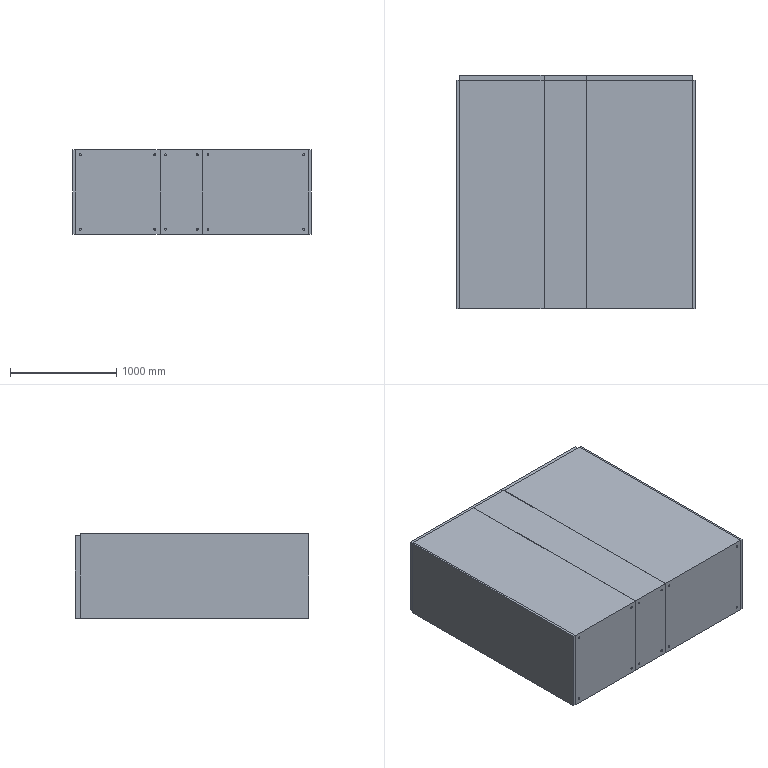Part | STEP file | 400-MC-101 | 5 solids | 238 faces | box 2242 x 2200 x 800 mm | volume 3938278879 mm3 | plane 155 | spline 59 | cylinder 24 | commonest cylinder face diameters 18 x24